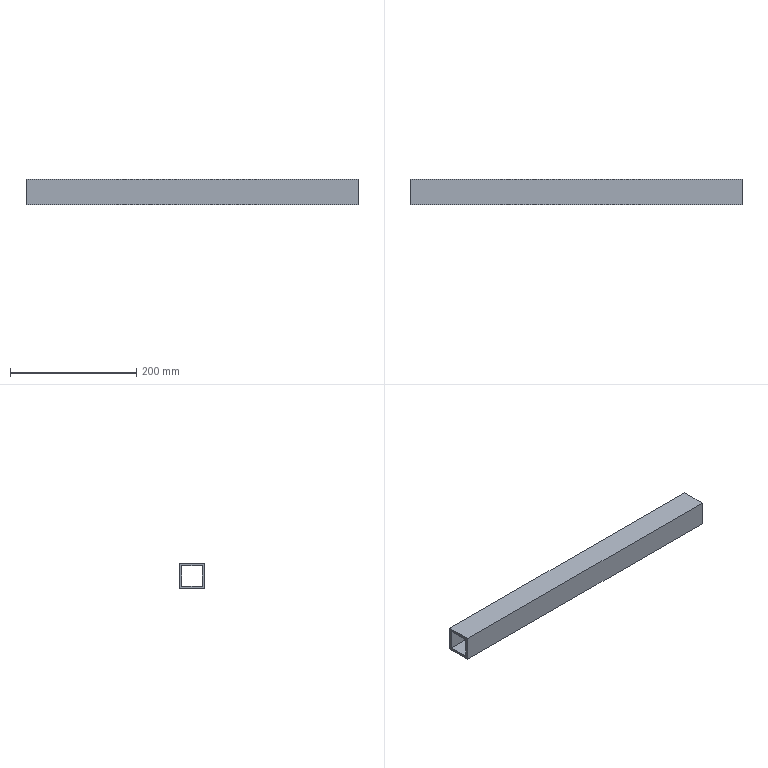Part | NX | features solid 2 | 1 solid | 10 faces | box 525 x 40 x 40 mm | volume 302400 mm3 | plane 10
STEP:
#1=CARTESIAN_POINT('',(-1180.,170.,-85.));
#2=VERTEX_POINT('',#1);
#3=CARTESIAN_POINT('',(-655.,170.,-85.));
#4=VERTEX_POINT('',#3);
#5=CARTESIAN_POINT('',(204.393,170.,-85.));
#6=DIRECTION('',(1.,0.,0.));
#7=VECTOR('',#6,1000.);
#8=LINE('',#5,#7);
#9=EDGE_CURVE('',#2,#4,#8,.T.);
#10=ORIENTED_EDGE('',*,*,#9,.F.);
#11=CARTESIAN_POINT('',(-1180.,170.,-45.));
#12=VERTEX_POINT('',#11);
#13=CARTESIAN_POINT('',(-1180.,170.,-40.));
#14=DIRECTION('',(0.,0.,1.));
#15=VECTOR('',#14,1000.);
#16=LINE('',#13,#15);
#17=EDGE_CURVE('',#2,#12,#16,.T.);
#18=ORIENTED_EDGE('',*,*,#17,.T.);
#19=CARTESIAN_POINT('',(-655.,170.,-45.));
#20=VERTEX_POINT('',#19);
#21=CARTESIAN_POINT('',(204.393,170.,-45.));
#22=DIRECTION('',(-1.,0.,0.));
#23=VECTOR('',#22,1000.);
#24=LINE('',#21,#23);
#25=EDGE_CURVE('',#20,#12,#24,.T.);
#26=ORIENTED_EDGE('',*,*,#25,.F.);
#27=CARTESIAN_POINT('',(-655.,170.,-40.));
#28=DIRECTION('',(0.,0.,1.));
#29=VECTOR('',#28,1000.);
#30=LINE('',#27,#29);
#31=EDGE_CURVE('',#4,#20,#30,.T.);
#32=ORIENTED_EDGE('',*,*,#31,.F.);
#33=EDGE_LOOP('',(#10,#18,#26,#32));
#34=FACE_BOUND('',#33,.T.);
#35=CARTESIAN_POINT('',(119.393,170.,-40.));
#36=DIRECTION('',(0.,-1.,0.));
#37=DIRECTION('',(0.,0.,-1.));
#38=AXIS2_PLACEMENT_3D('',#35,#36,#37);
#39=PLANE('',#38);
#40=ADVANCED_FACE('',(#34),#39,.F.);
#41=ORIENTED_EDGE('',*,*,#25,.T.);
#42=CARTESIAN_POINT('',(-1180.,130.,-45.));
#43=VERTEX_POINT('',#42);
#44=CARTESIAN_POINT('',(-1180.,-490.,-45.));
#45=DIRECTION('',(0.,-1.,0.));
#46=VECTOR('',#45,1000.);
#47=LINE('',#44,#46);
#48=EDGE_CURVE('',#12,#43,#47,.T.);
#49=ORIENTED_EDGE('',*,*,#48,.T.);
#50=CARTESIAN_POINT('',(-655.,130.,-45.));
#51=VERTEX_POINT('',#50);
#52=CARTESIAN_POINT('',(204.393,130.,-45.));
#53=DIRECTION('',(1.,0.,0.));
#54=VECTOR('',#53,1000.);
#55=LINE('',#52,#54);
#56=EDGE_CURVE('',#43,#51,#55,.T.);
#57=ORIENTED_EDGE('',*,*,#56,.T.);
#58=CARTESIAN_POINT('',(-655.,-490.,-45.));
#59=DIRECTION('',(0.,-1.,0.));
#60=VECTOR('',#59,1000.);
#61=LINE('',#58,#60);
#62=EDGE_CURVE('',#20,#51,#61,.T.);
#63=ORIENTED_EDGE('',*,*,#62,.F.);
#64=EDGE_LOOP('',(#41,#49,#57,#63));
#65=FACE_BOUND('',#64,.T.);
#66=CARTESIAN_POINT('',(204.393,-490.,-45.));
#67=DIRECTION('',(0.,0.,-1.));
#68=DIRECTION('',(0.,1.,0.));
#69=AXIS2_PLACEMENT_3D('',#66,#67,#68);
#70=PLANE('',#69);
#71=ADVANCED_FACE('',(#65),#70,.F.);
#72=CARTESIAN_POINT('',(-1180.,130.,-85.));
#73=VERTEX_POINT('',#72);
#74=CARTESIAN_POINT('',(-655.,130.,-85.));
#75=VERTEX_POINT('',#74);
#76=CARTESIAN_POINT('',(119.393,130.,-85.));
#77=DIRECTION('',(1.,0.,0.));
#78=VECTOR('',#77,1000.);
#79=LINE('',#76,#78);
#80=EDGE_CURVE('',#73,#75,#79,.T.);
#81=ORIENTED_EDGE('',*,*,#80,.F.);
#82=CARTESIAN_POINT('',(-1180.,-450.,-85.));
#83=DIRECTION('',(0.,1.,0.));
#84=VECTOR('',#83,1000.);
#85=LINE('',#82,#84);
#86=EDGE_CURVE('',#73,#2,#85,.T.);
#87=ORIENTED_EDGE('',*,*,#86,.T.);
#88=ORIENTED_EDGE('',*,*,#9,.T.);
#89=CARTESIAN_POINT('',(-655.,-450.,-85.));
#90=DIRECTION('',(0.,1.,0.));
#91=VECTOR('',#90,1000.);
#92=LINE('',#89,#91);
#93=EDGE_CURVE('',#75,#4,#92,.T.);
#94=ORIENTED_EDGE('',*,*,#93,.F.);
#95=EDGE_LOOP('',(#81,#87,#88,#94));
#96=FACE_BOUND('',#95,.T.);
#97=CARTESIAN_POINT('',(204.393,-450.,-85.));
#98=DIRECTION('',(0.,0.,1.));
#99=DIRECTION('',(0.,-1.,0.));
#100=AXIS2_PLACEMENT_3D('',#97,#98,#99);
#101=PLANE('',#100);
#102=ADVANCED_FACE('',(#96),#101,.F.);
#103=ORIENTED_EDGE('',*,*,#56,.F.);
#104=CARTESIAN_POINT('',(-1180.,130.,-70.));
#105=DIRECTION('',(0.,0.,-1.));
#106=VECTOR('',#105,1000.);
#107=LINE('',#104,#106);
#108=EDGE_CURVE('',#43,#73,#107,.T.);
#109=ORIENTED_EDGE('',*,*,#108,.T.);
#110=ORIENTED_EDGE('',*,*,#80,.T.);
#111=CARTESIAN_POINT('',(-655.,130.,-70.));
#112=DIRECTION('',(0.,0.,-1.));
#113=VECTOR('',#112,1000.);
#114=LINE('',#111,#113);
#115=EDGE_CURVE('',#51,#75,#114,.T.);
#116=ORIENTED_EDGE('',*,*,#115,.F.);
#117=EDGE_LOOP('',(#103,#109,#110,#116));
#118=FACE_BOUND('',#117,.T.);
#119=CARTESIAN_POINT('',(119.393,130.,-70.));
#120=DIRECTION('',(0.,1.,0.));
#121=DIRECTION('',(0.,0.,1.));
#122=AXIS2_PLACEMENT_3D('',#119,#120,#121);
#123=PLANE('',#122);
#124=ADVANCED_FACE('',(#118),#123,.F.);
#125=CARTESIAN_POINT('',(-1180.,166.,-81.));
#126=VERTEX_POINT('',#125);
#127=CARTESIAN_POINT('',(-1180.,166.,-49.));
#128=VERTEX_POINT('',#127);
#129=CARTESIAN_POINT('',(-1180.,166.,-40.));
#130=DIRECTION('',(0.,0.,1.));
#131=VECTOR('',#130,1000.);
#132=LINE('',#129,#131);
#133=EDGE_CURVE('',#126,#128,#132,.T.);
#134=ORIENTED_EDGE('',*,*,#133,.F.);
#135=CARTESIAN_POINT('',(-655.,166.,-81.));
#136=VERTEX_POINT('',#135);
#137=CARTESIAN_POINT('',(204.393,166.,-81.));
#138=DIRECTION('',(1.,0.,0.));
#139=VECTOR('',#138,1000.);
#140=LINE('',#137,#139);
#141=EDGE_CURVE('',#126,#136,#140,.T.);
#142=ORIENTED_EDGE('',*,*,#141,.T.);
#143=CARTESIAN_POINT('',(-655.,166.,-49.));
#144=VERTEX_POINT('',#143);
#145=CARTESIAN_POINT('',(-655.,166.,-40.));
#146=DIRECTION('',(0.,0.,1.));
#147=VECTOR('',#146,1000.);
#148=LINE('',#145,#147);
#149=EDGE_CURVE('',#136,#144,#148,.T.);
#150=ORIENTED_EDGE('',*,*,#149,.T.);
#151=CARTESIAN_POINT('',(204.393,166.,-49.));
#152=DIRECTION('',(-1.,0.,0.));
#153=VECTOR('',#152,1000.);
#154=LINE('',#151,#153);
#155=EDGE_CURVE('',#144,#128,#154,.T.);
#156=ORIENTED_EDGE('',*,*,#155,.T.);
#157=EDGE_LOOP('',(#134,#142,#150,#156));
#158=FACE_BOUND('',#157,.T.);
#159=CARTESIAN_POINT('',(119.393,166.,-40.));
#160=DIRECTION('',(0.,-1.,0.));
#161=DIRECTION('',(0.,0.,-1.));
#162=AXIS2_PLACEMENT_3D('',#159,#160,#161);
#163=PLANE('',#162);
#164=ADVANCED_FACE('',(#158),#163,.T.);
#165=CARTESIAN_POINT('',(-1180.,134.,-49.));
#166=VERTEX_POINT('',#165);
#167=CARTESIAN_POINT('',(-1180.,-490.,-49.));
#168=DIRECTION('',(0.,-1.,0.));
#169=VECTOR('',#168,1000.);
#170=LINE('',#167,#169);
#171=EDGE_CURVE('',#128,#166,#170,.T.);
#172=ORIENTED_EDGE('',*,*,#171,.F.);
#173=ORIENTED_EDGE('',*,*,#155,.F.);
#174=CARTESIAN_POINT('',(-655.,134.,-49.));
#175=VERTEX_POINT('',#174);
#176=CARTESIAN_POINT('',(-655.,-490.,-49.));
#177=DIRECTION('',(0.,-1.,0.));
#178=VECTOR('',#177,1000.);
#179=LINE('',#176,#178);
#180=EDGE_CURVE('',#144,#175,#179,.T.);
#181=ORIENTED_EDGE('',*,*,#180,.T.);
#182=CARTESIAN_POINT('',(204.393,134.,-49.));
#183=DIRECTION('',(1.,0.,0.));
#184=VECTOR('',#183,1000.);
#185=LINE('',#182,#184);
#186=EDGE_CURVE('',#166,#175,#185,.T.);
#187=ORIENTED_EDGE('',*,*,#186,.F.);
#188=EDGE_LOOP('',(#172,#173,#181,#187));
#189=FACE_BOUND('',#188,.T.);
#190=CARTESIAN_POINT('',(204.393,-490.,-49.));
#191=DIRECTION('',(0.,0.,-1.));
#192=DIRECTION('',(0.,1.,0.));
#193=AXIS2_PLACEMENT_3D('',#190,#191,#192);
#194=PLANE('',#193);
#195=ADVANCED_FACE('',(#189),#194,.T.);
#196=CARTESIAN_POINT('',(-1180.,134.,-81.));
#197=VERTEX_POINT('',#196);
#198=CARTESIAN_POINT('',(-1180.,-450.,-81.));
#199=DIRECTION('',(0.,1.,0.));
#200=VECTOR('',#199,1000.);
#201=LINE('',#198,#200);
#202=EDGE_CURVE('',#197,#126,#201,.T.);
#203=ORIENTED_EDGE('',*,*,#202,.F.);
#204=CARTESIAN_POINT('',(-655.,134.,-81.));
#205=VERTEX_POINT('',#204);
#206=CARTESIAN_POINT('',(119.393,134.,-81.));
#207=DIRECTION('',(1.,0.,0.));
#208=VECTOR('',#207,1000.);
#209=LINE('',#206,#208);
#210=EDGE_CURVE('',#197,#205,#209,.T.);
#211=ORIENTED_EDGE('',*,*,#210,.T.);
#212=CARTESIAN_POINT('',(-655.,-450.,-81.));
#213=DIRECTION('',(0.,1.,0.));
#214=VECTOR('',#213,1000.);
#215=LINE('',#212,#214);
#216=EDGE_CURVE('',#205,#136,#215,.T.);
#217=ORIENTED_EDGE('',*,*,#216,.T.);
#218=ORIENTED_EDGE('',*,*,#141,.F.);
#219=EDGE_LOOP('',(#203,#211,#217,#218));
#220=FACE_BOUND('',#219,.T.);
#221=CARTESIAN_POINT('',(204.393,-450.,-81.));
#222=DIRECTION('',(0.,0.,1.));
#223=DIRECTION('',(0.,-1.,0.));
#224=AXIS2_PLACEMENT_3D('',#221,#222,#223);
#225=PLANE('',#224);
#226=ADVANCED_FACE('',(#220),#225,.T.);
#227=CARTESIAN_POINT('',(-1180.,134.,-70.));
#228=DIRECTION('',(0.,0.,-1.));
#229=VECTOR('',#228,1000.);
#230=LINE('',#227,#229);
#231=EDGE_CURVE('',#166,#197,#230,.T.);
#232=ORIENTED_EDGE('',*,*,#231,.F.);
#233=ORIENTED_EDGE('',*,*,#186,.T.);
#234=CARTESIAN_POINT('',(-655.,134.,-70.));
#235=DIRECTION('',(0.,0.,-1.));
#236=VECTOR('',#235,1000.);
#237=LINE('',#234,#236);
#238=EDGE_CURVE('',#175,#205,#237,.T.);
#239=ORIENTED_EDGE('',*,*,#238,.T.);
#240=ORIENTED_EDGE('',*,*,#210,.F.);
#241=EDGE_LOOP('',(#232,#233,#239,#240));
#242=FACE_BOUND('',#241,.T.);
#243=CARTESIAN_POINT('',(119.393,134.,-70.));
#244=DIRECTION('',(0.,1.,0.));
#245=DIRECTION('',(0.,0.,1.));
#246=AXIS2_PLACEMENT_3D('',#243,#244,#245);
#247=PLANE('',#246);
#248=ADVANCED_FACE('',(#242),#247,.T.);
#249=ORIENTED_EDGE('',*,*,#149,.F.);
#250=ORIENTED_EDGE('',*,*,#216,.F.);
#251=ORIENTED_EDGE('',*,*,#238,.F.);
#252=ORIENTED_EDGE('',*,*,#180,.F.);
#253=EDGE_LOOP('',(#249,#250,#251,#252));
#254=FACE_BOUND('',#253,.T.);
#255=ORIENTED_EDGE('',*,*,#93,.T.);
#256=ORIENTED_EDGE('',*,*,#31,.T.);
#257=ORIENTED_EDGE('',*,*,#62,.T.);
#258=ORIENTED_EDGE('',*,*,#115,.T.);
#259=EDGE_LOOP('',(#255,#256,#257,#258));
#260=FACE_BOUND('',#259,.T.);
#261=CARTESIAN_POINT('',(-655.,159.6,-24.));
#262=DIRECTION('',(1.,0.,0.));
#263=DIRECTION('',(0.,0.,-1.));
#264=AXIS2_PLACEMENT_3D('',#261,#262,#263);
#265=PLANE('',#264);
#266=ADVANCED_FACE('',(#254,#260),#265,.T.);
#267=ORIENTED_EDGE('',*,*,#133,.T.);
#268=ORIENTED_EDGE('',*,*,#171,.T.);
#269=ORIENTED_EDGE('',*,*,#231,.T.);
#270=ORIENTED_EDGE('',*,*,#202,.T.);
#271=EDGE_LOOP('',(#267,#268,#269,#270));
#272=FACE_BOUND('',#271,.T.);
#273=ORIENTED_EDGE('',*,*,#86,.F.);
#274=ORIENTED_EDGE('',*,*,#108,.F.);
#275=ORIENTED_EDGE('',*,*,#48,.F.);
#276=ORIENTED_EDGE('',*,*,#17,.F.);
#277=EDGE_LOOP('',(#273,#274,#275,#276));
#278=FACE_BOUND('',#277,.T.);
#279=CARTESIAN_POINT('',(-1180.,-180.,-45.));
#280=DIRECTION('',(1.,0.,0.));
#281=DIRECTION('',(0.,0.,-1.));
#282=AXIS2_PLACEMENT_3D('',#279,#280,#281);
#283=PLANE('',#282);
#284=ADVANCED_FACE('',(#272,#278),#283,.F.);
#285=CLOSED_SHELL('',(#40,#71,#102,#124,#164,#195,#226,#248,#266,#284));
#286=MANIFOLD_SOLID_BREP('',#285);
#287=(LENGTH_UNIT()NAMED_UNIT(*)SI_UNIT(.MILLI.,.METRE.));
#288=UNCERTAINTY_MEASURE_WITH_UNIT(LENGTH_MEASURE(0.00001),#287,'','');
#289=(NAMED_UNIT(*)PLANE_ANGLE_UNIT()SI_UNIT($,.RADIAN.));
#290=(NAMED_UNIT(*)SI_UNIT($,.STERADIAN.)SOLID_ANGLE_UNIT());
#291=(GEOMETRIC_REPRESENTATION_CONTEXT(3)GLOBAL_UNCERTAINTY_ASSIGNED_CONTEXT((#288))GLOBAL_UNIT_ASSIGNED_CONTEXT((#287,#289,#290))REPRESENTATION_CONTEXT('',''));
#292=ADVANCED_BREP_SHAPE_REPRESENTATION('',(#286),#291);